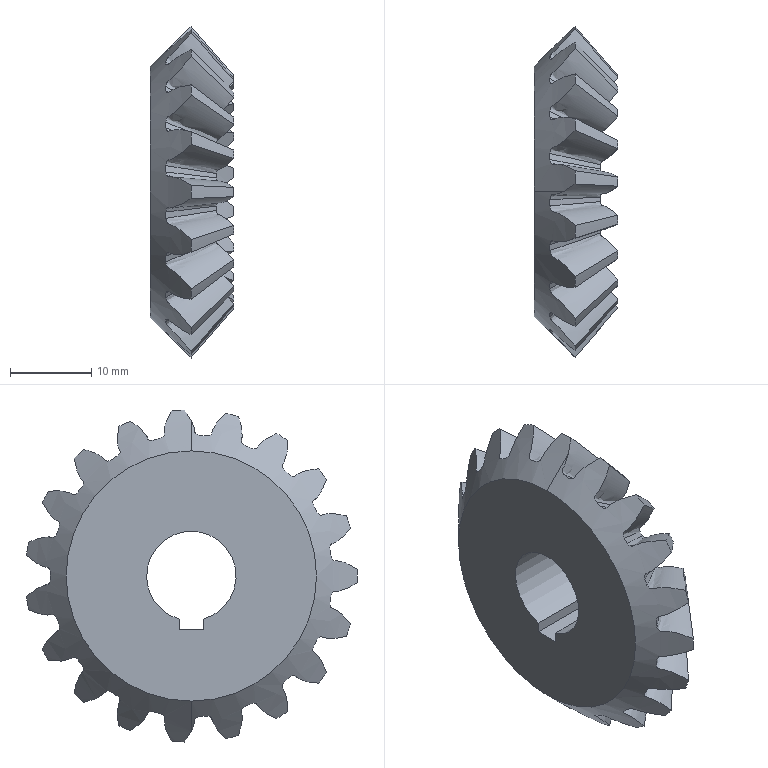Part | SolidWorks | features 3DProfileFeature 12, ICE 2, BlendCut 1, CirPattern 1, RefAxis 1, Revolution 1 | 1 solid | 86 faces | box 10.311 x 40.668 x 40.791 mm | volume 6619 mm3 | spline 38 | plane 24 | cone 23 | cylinder 1 | commonest cylinder face diameters 11 x1